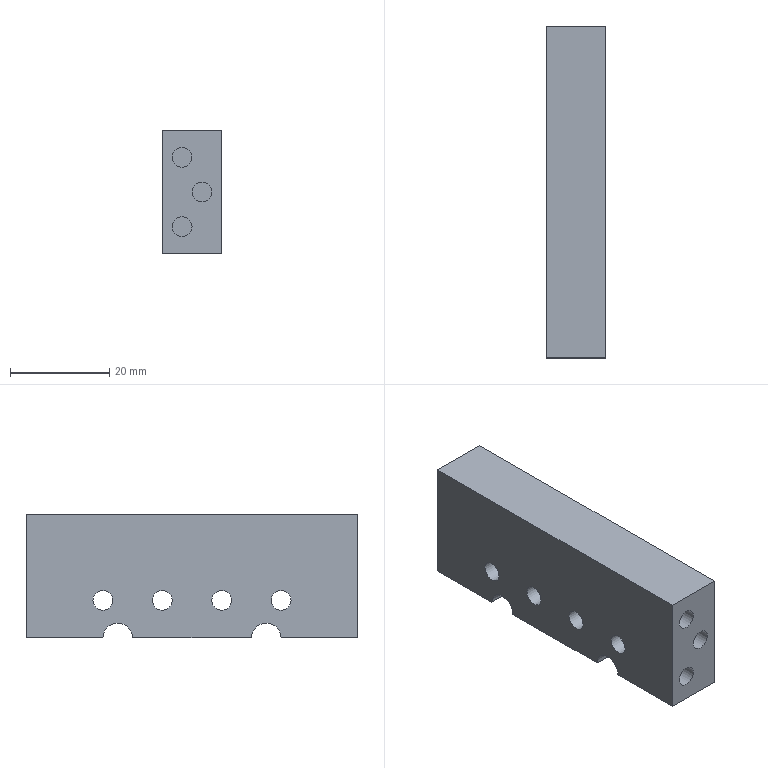Part | STEP file | 1-01.3 | 1 solid | 28 faces | box 12 x 67 x 25 mm | volume 18121 mm3 | plane 15 | cylinder 13 | commonest cylinder face diameters 4 x10 6 x3